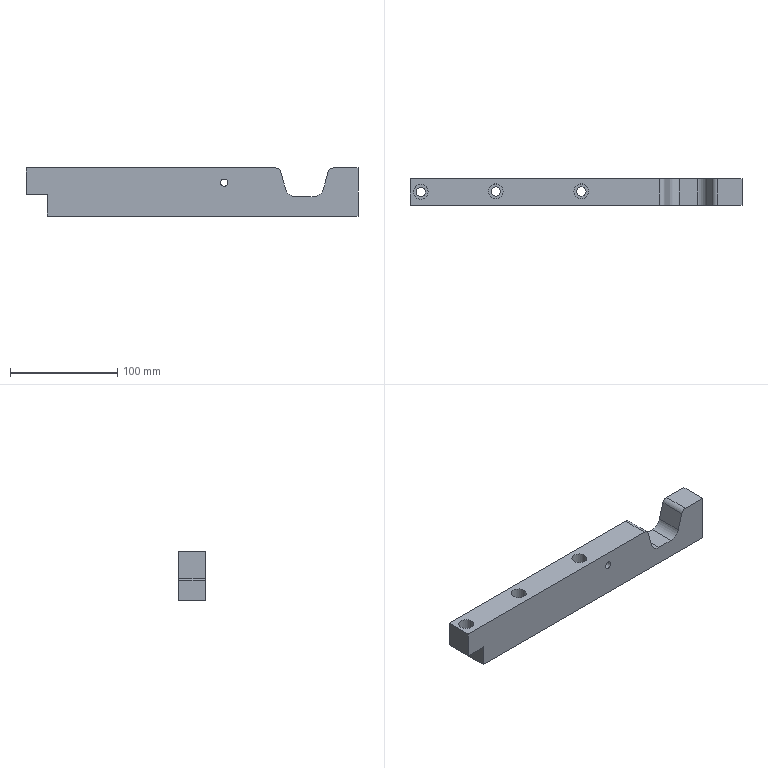Part | STEP file | YBQDJ-FLJ-4 | 1 solid | 30 faces | box 310 x 25 x 45 mm | volume 300462 mm3 | plane 15 | cylinder 14 | cone 1 | commonest cylinder face diameters 8.7 x3 14 x3 4 x2 10 x2 20 x2 1 x1